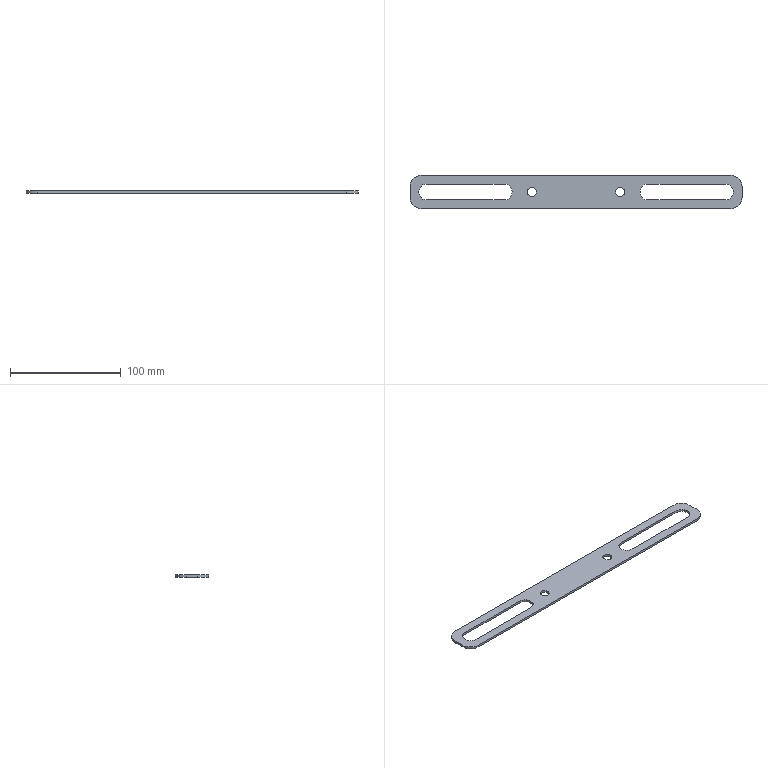Part | SolidWorks | features Fillet 2, ICE 2, Extrusion 1, MirrorPattern 1 | 1 solid | 24 faces | box 300 x 30 x 2 mm | volume 12944 mm3 | cylinder 14 | plane 10 | commonest cylinder face diameters 14.4 x6 8 x4 20 x4
STEP:
#1=CARTESIAN_POINT('',(44.,0.,2.));
#2=VERTEX_POINT('',#1);
#3=CARTESIAN_POINT('',(36.,0.,2.));
#4=VERTEX_POINT('',#3);
#5=CARTESIAN_POINT('',(40.,0.,2.));
#6=DIRECTION('',(0.,0.,-1.));
#7=DIRECTION('',(-1.,0.,0.));
#8=AXIS2_PLACEMENT_3D('',#5,#6,#7);
#9=CIRCLE('',#8,4.);
#10=EDGE_CURVE('',#2,#4,#9,.T.);
#11=ORIENTED_EDGE('',*,*,#10,.F.);
#12=CARTESIAN_POINT('',(44.,0.,0.));
#13=VERTEX_POINT('',#12);
#14=CARTESIAN_POINT('',(44.,0.,2.));
#15=DIRECTION('',(0.,0.,-1.));
#16=VECTOR('',#15,1000.);
#17=LINE('',#14,#16);
#18=EDGE_CURVE('',#2,#13,#17,.T.);
#19=ORIENTED_EDGE('',*,*,#18,.T.);
#20=CARTESIAN_POINT('',(36.,0.,0.));
#21=VERTEX_POINT('',#20);
#22=CARTESIAN_POINT('',(40.,0.,0.));
#23=DIRECTION('',(0.,0.,-1.));
#24=DIRECTION('',(-1.,0.,0.));
#25=AXIS2_PLACEMENT_3D('',#22,#23,#24);
#26=CIRCLE('',#25,4.);
#27=EDGE_CURVE('',#13,#21,#26,.T.);
#28=ORIENTED_EDGE('',*,*,#27,.T.);
#29=CARTESIAN_POINT('',(36.,0.,2.));
#30=DIRECTION('',(0.,0.,-1.));
#31=VECTOR('',#30,1000.);
#32=LINE('',#29,#31);
#33=EDGE_CURVE('',#4,#21,#32,.T.);
#34=ORIENTED_EDGE('',*,*,#33,.F.);
#35=EDGE_LOOP('',(#11,#19,#28,#34));
#36=FACE_OUTER_BOUND('',#35,.T.);
#37=CARTESIAN_POINT('',(40.,0.,2.));
#38=DIRECTION('',(0.,0.,-1.));
#39=DIRECTION('',(-1.,0.,0.));
#40=AXIS2_PLACEMENT_3D('',#37,#38,#39);
#41=CYLINDRICAL_SURFACE('',#40,4.);
#42=ADVANCED_FACE('',(#36),#41,.F.);
#43=CARTESIAN_POINT('',(-36.,0.,2.));
#44=VERTEX_POINT('',#43);
#45=CARTESIAN_POINT('',(-44.,0.,2.));
#46=VERTEX_POINT('',#45);
#47=CARTESIAN_POINT('',(-40.,0.,2.));
#48=DIRECTION('',(0.,0.,-1.));
#49=DIRECTION('',(-1.,0.,0.));
#50=AXIS2_PLACEMENT_3D('',#47,#48,#49);
#51=CIRCLE('',#50,4.);
#52=EDGE_CURVE('',#44,#46,#51,.T.);
#53=ORIENTED_EDGE('',*,*,#52,.F.);
#54=CARTESIAN_POINT('',(-36.,0.,0.));
#55=VERTEX_POINT('',#54);
#56=CARTESIAN_POINT('',(-36.,0.,2.));
#57=DIRECTION('',(0.,0.,-1.));
#58=VECTOR('',#57,1000.);
#59=LINE('',#56,#58);
#60=EDGE_CURVE('',#44,#55,#59,.T.);
#61=ORIENTED_EDGE('',*,*,#60,.T.);
#62=CARTESIAN_POINT('',(-44.,0.,0.));
#63=VERTEX_POINT('',#62);
#64=CARTESIAN_POINT('',(-40.,0.,0.));
#65=DIRECTION('',(0.,0.,-1.));
#66=DIRECTION('',(-1.,0.,0.));
#67=AXIS2_PLACEMENT_3D('',#64,#65,#66);
#68=CIRCLE('',#67,4.);
#69=EDGE_CURVE('',#55,#63,#68,.T.);
#70=ORIENTED_EDGE('',*,*,#69,.T.);
#71=CARTESIAN_POINT('',(-44.,0.,2.));
#72=DIRECTION('',(0.,0.,-1.));
#73=VECTOR('',#72,1000.);
#74=LINE('',#71,#73);
#75=EDGE_CURVE('',#46,#63,#74,.T.);
#76=ORIENTED_EDGE('',*,*,#75,.F.);
#77=EDGE_LOOP('',(#53,#61,#70,#76));
#78=FACE_OUTER_BOUND('',#77,.T.);
#79=CARTESIAN_POINT('',(-40.,0.,2.));
#80=DIRECTION('',(0.,0.,-1.));
#81=DIRECTION('',(-1.,0.,0.));
#82=AXIS2_PLACEMENT_3D('',#79,#80,#81);
#83=CYLINDRICAL_SURFACE('',#82,4.);
#84=ADVANCED_FACE('',(#78),#83,.F.);
#85=CARTESIAN_POINT('',(135.,7.2,0.));
#86=VERTEX_POINT('',#85);
#87=CARTESIAN_POINT('',(142.2,0.,0.));
#88=VERTEX_POINT('',#87);
#89=CARTESIAN_POINT('',(135.,0.,0.));
#90=DIRECTION('',(0.,0.,-1.));
#91=DIRECTION('',(-1.,0.,0.));
#92=AXIS2_PLACEMENT_3D('',#89,#90,#91);
#93=CIRCLE('',#92,7.2);
#94=EDGE_CURVE('',#86,#88,#93,.T.);
#95=ORIENTED_EDGE('',*,*,#94,.T.);
#96=CARTESIAN_POINT('',(142.2,0.,2.));
#97=VERTEX_POINT('',#96);
#98=CARTESIAN_POINT('',(142.2,0.,0.));
#99=DIRECTION('',(0.,0.,1.));
#100=VECTOR('',#99,1000.);
#101=LINE('',#98,#100);
#102=EDGE_CURVE('',#88,#97,#101,.T.);
#103=ORIENTED_EDGE('',*,*,#102,.T.);
#104=CARTESIAN_POINT('',(135.,7.2,2.));
#105=VERTEX_POINT('',#104);
#106=CARTESIAN_POINT('',(135.,0.,2.));
#107=DIRECTION('',(0.,0.,-1.));
#108=DIRECTION('',(-1.,0.,0.));
#109=AXIS2_PLACEMENT_3D('',#106,#107,#108);
#110=CIRCLE('',#109,7.2);
#111=EDGE_CURVE('',#105,#97,#110,.T.);
#112=ORIENTED_EDGE('',*,*,#111,.F.);
#113=CARTESIAN_POINT('',(135.,7.2,0.));
#114=DIRECTION('',(0.,0.,1.));
#115=VECTOR('',#114,1000.);
#116=LINE('',#113,#115);
#117=EDGE_CURVE('',#86,#105,#116,.T.);
#118=ORIENTED_EDGE('',*,*,#117,.F.);
#119=EDGE_LOOP('',(#95,#103,#112,#118));
#120=FACE_OUTER_BOUND('',#119,.T.);
#121=CARTESIAN_POINT('',(135.,0.,0.));
#122=DIRECTION('',(0.,0.,1.));
#123=DIRECTION('',(1.,0.,0.));
#124=AXIS2_PLACEMENT_3D('',#121,#122,#123);
#125=CYLINDRICAL_SURFACE('',#124,7.2);
#126=ADVANCED_FACE('',(#120),#125,.F.);
#127=CARTESIAN_POINT('',(-57.8,0.,0.));
#128=VERTEX_POINT('',#127);
#129=CARTESIAN_POINT('',(-65.,7.2,0.));
#130=VERTEX_POINT('',#129);
#131=CARTESIAN_POINT('',(-65.,0.,0.));
#132=DIRECTION('',(0.,0.,1.));
#133=DIRECTION('',(1.,0.,0.));
#134=AXIS2_PLACEMENT_3D('',#131,#132,#133);
#135=CIRCLE('',#134,7.2);
#136=EDGE_CURVE('',#128,#130,#135,.T.);
#137=ORIENTED_EDGE('',*,*,#136,.F.);
#138=CARTESIAN_POINT('',(-57.8,0.,2.));
#139=VERTEX_POINT('',#138);
#140=CARTESIAN_POINT('',(-57.8,0.,0.));
#141=DIRECTION('',(0.,0.,1.));
#142=VECTOR('',#141,1000.);
#143=LINE('',#140,#142);
#144=EDGE_CURVE('',#128,#139,#143,.T.);
#145=ORIENTED_EDGE('',*,*,#144,.T.);
#146=CARTESIAN_POINT('',(-65.,7.2,2.));
#147=VERTEX_POINT('',#146);
#148=CARTESIAN_POINT('',(-65.,0.,2.));
#149=DIRECTION('',(0.,0.,1.));
#150=DIRECTION('',(1.,0.,0.));
#151=AXIS2_PLACEMENT_3D('',#148,#149,#150);
#152=CIRCLE('',#151,7.2);
#153=EDGE_CURVE('',#139,#147,#152,.T.);
#154=ORIENTED_EDGE('',*,*,#153,.T.);
#155=CARTESIAN_POINT('',(-65.,7.2,0.));
#156=DIRECTION('',(0.,0.,1.));
#157=VECTOR('',#156,1000.);
#158=LINE('',#155,#157);
#159=EDGE_CURVE('',#130,#147,#158,.T.);
#160=ORIENTED_EDGE('',*,*,#159,.F.);
#161=EDGE_LOOP('',(#137,#145,#154,#160));
#162=FACE_OUTER_BOUND('',#161,.T.);
#163=CARTESIAN_POINT('',(-65.,0.,0.));
#164=DIRECTION('',(0.,0.,1.));
#165=DIRECTION('',(1.,0.,0.));
#166=AXIS2_PLACEMENT_3D('',#163,#164,#165);
#167=CYLINDRICAL_SURFACE('',#166,7.2);
#168=ADVANCED_FACE('',(#162),#167,.F.);
#169=CARTESIAN_POINT('',(40.,0.,2.));
#170=DIRECTION('',(0.,0.,-1.));
#171=DIRECTION('',(-1.,0.,0.));
#172=AXIS2_PLACEMENT_3D('',#169,#170,#171);
#173=CIRCLE('',#172,4.);
#174=EDGE_CURVE('',#4,#2,#173,.T.);
#175=ORIENTED_EDGE('',*,*,#174,.T.);
#176=ORIENTED_EDGE('',*,*,#10,.T.);
#177=EDGE_LOOP('',(#175,#176));
#178=FACE_BOUND('',#177,.T.);
#179=CARTESIAN_POINT('',(-40.,0.,2.));
#180=DIRECTION('',(0.,0.,-1.));
#181=DIRECTION('',(-1.,0.,0.));
#182=AXIS2_PLACEMENT_3D('',#179,#180,#181);
#183=CIRCLE('',#182,4.);
#184=EDGE_CURVE('',#46,#44,#183,.T.);
#185=ORIENTED_EDGE('',*,*,#184,.T.);
#186=ORIENTED_EDGE('',*,*,#52,.T.);
#187=EDGE_LOOP('',(#185,#186));
#188=FACE_BOUND('',#187,.T.);
#189=CARTESIAN_POINT('',(-140.,-15.,2.));
#190=VERTEX_POINT('',#189);
#191=CARTESIAN_POINT('',(140.,-15.,2.));
#192=VERTEX_POINT('',#191);
#193=CARTESIAN_POINT('',(150.,-15.,2.));
#194=DIRECTION('',(1.,0.,0.));
#195=VECTOR('',#194,1000.);
#196=LINE('',#193,#195);
#197=EDGE_CURVE('',#190,#192,#196,.T.);
#198=ORIENTED_EDGE('',*,*,#197,.T.);
#199=CARTESIAN_POINT('',(150.,-5.,2.));
#200=VERTEX_POINT('',#199);
#201=CARTESIAN_POINT('',(140.,-5.,2.));
#202=DIRECTION('',(0.,0.,1.));
#203=DIRECTION('',(1.,0.,0.));
#204=AXIS2_PLACEMENT_3D('',#201,#202,#203);
#205=CIRCLE('',#204,10.);
#206=EDGE_CURVE('',#192,#200,#205,.T.);
#207=ORIENTED_EDGE('',*,*,#206,.T.);
#208=CARTESIAN_POINT('',(150.,5.,2.));
#209=VERTEX_POINT('',#208);
#210=CARTESIAN_POINT('',(150.,-15.,2.));
#211=DIRECTION('',(0.,1.,0.));
#212=VECTOR('',#211,1000.);
#213=LINE('',#210,#212);
#214=EDGE_CURVE('',#200,#209,#213,.T.);
#215=ORIENTED_EDGE('',*,*,#214,.T.);
#216=CARTESIAN_POINT('',(140.,15.,2.));
#217=VERTEX_POINT('',#216);
#218=CARTESIAN_POINT('',(140.,5.,2.));
#219=DIRECTION('',(0.,0.,1.));
#220=DIRECTION('',(1.,0.,0.));
#221=AXIS2_PLACEMENT_3D('',#218,#219,#220);
#222=CIRCLE('',#221,10.);
#223=EDGE_CURVE('',#209,#217,#222,.T.);
#224=ORIENTED_EDGE('',*,*,#223,.T.);
#225=CARTESIAN_POINT('',(-140.,15.,2.));
#226=VERTEX_POINT('',#225);
#227=CARTESIAN_POINT('',(150.,15.,2.));
#228=DIRECTION('',(-1.,0.,0.));
#229=VECTOR('',#228,1000.);
#230=LINE('',#227,#229);
#231=EDGE_CURVE('',#217,#226,#230,.T.);
#232=ORIENTED_EDGE('',*,*,#231,.T.);
#233=CARTESIAN_POINT('',(-150.,5.,2.));
#234=VERTEX_POINT('',#233);
#235=CARTESIAN_POINT('',(-140.,5.,2.));
#236=DIRECTION('',(0.,0.,1.));
#237=DIRECTION('',(1.,0.,0.));
#238=AXIS2_PLACEMENT_3D('',#235,#236,#237);
#239=CIRCLE('',#238,10.);
#240=EDGE_CURVE('',#226,#234,#239,.T.);
#241=ORIENTED_EDGE('',*,*,#240,.T.);
#242=CARTESIAN_POINT('',(-150.,-5.,2.));
#243=VERTEX_POINT('',#242);
#244=CARTESIAN_POINT('',(-150.,-15.,2.));
#245=DIRECTION('',(0.,-1.,0.));
#246=VECTOR('',#245,1000.);
#247=LINE('',#244,#246);
#248=EDGE_CURVE('',#234,#243,#247,.T.);
#249=ORIENTED_EDGE('',*,*,#248,.T.);
#250=CARTESIAN_POINT('',(-140.,-5.,2.));
#251=DIRECTION('',(0.,0.,1.));
#252=DIRECTION('',(1.,0.,0.));
#253=AXIS2_PLACEMENT_3D('',#250,#251,#252);
#254=CIRCLE('',#253,10.);
#255=EDGE_CURVE('',#243,#190,#254,.T.);
#256=ORIENTED_EDGE('',*,*,#255,.T.);
#257=EDGE_LOOP('',(#198,#207,#215,#224,#232,#241,#249,#256));
#258=FACE_OUTER_BOUND('',#257,.T.);
#259=CARTESIAN_POINT('',(-135.,7.2,2.));
#260=VERTEX_POINT('',#259);
#261=CARTESIAN_POINT('',(-135.,-7.2,2.));
#262=VERTEX_POINT('',#261);
#263=CARTESIAN_POINT('',(-135.,0.,2.));
#264=DIRECTION('',(0.,0.,1.));
#265=DIRECTION('',(1.,0.,0.));
#266=AXIS2_PLACEMENT_3D('',#263,#264,#265);
#267=CIRCLE('',#266,7.2);
#268=EDGE_CURVE('',#260,#262,#267,.T.);
#269=ORIENTED_EDGE('',*,*,#268,.F.);
#270=CARTESIAN_POINT('',(-135.,7.2,2.));
#271=DIRECTION('',(-1.,0.,0.));
#272=VECTOR('',#271,1000.);
#273=LINE('',#270,#272);
#274=EDGE_CURVE('',#147,#260,#273,.T.);
#275=ORIENTED_EDGE('',*,*,#274,.F.);
#276=ORIENTED_EDGE('',*,*,#153,.F.);
#277=CARTESIAN_POINT('',(-65.,-7.2,2.));
#278=VERTEX_POINT('',#277);
#279=CARTESIAN_POINT('',(-65.,0.,2.));
#280=DIRECTION('',(0.,0.,1.));
#281=DIRECTION('',(1.,0.,0.));
#282=AXIS2_PLACEMENT_3D('',#279,#280,#281);
#283=CIRCLE('',#282,7.2);
#284=EDGE_CURVE('',#278,#139,#283,.T.);
#285=ORIENTED_EDGE('',*,*,#284,.F.);
#286=CARTESIAN_POINT('',(-135.,-7.2,2.));
#287=DIRECTION('',(1.,0.,0.));
#288=VECTOR('',#287,1000.);
#289=LINE('',#286,#288);
#290=EDGE_CURVE('',#262,#278,#289,.T.);
#291=ORIENTED_EDGE('',*,*,#290,.F.);
#292=EDGE_LOOP('',(#269,#275,#276,#285,#291));
#293=FACE_BOUND('',#292,.T.);
#294=CARTESIAN_POINT('',(65.,7.2,2.));
#295=VERTEX_POINT('',#294);
#296=CARTESIAN_POINT('',(135.,7.2,2.));
#297=DIRECTION('',(1.,0.,0.));
#298=VECTOR('',#297,1000.);
#299=LINE('',#296,#298);
#300=EDGE_CURVE('',#295,#105,#299,.T.);
#301=ORIENTED_EDGE('',*,*,#300,.T.);
#302=ORIENTED_EDGE('',*,*,#111,.T.);
#303=CARTESIAN_POINT('',(135.,-7.2,2.));
#304=VERTEX_POINT('',#303);
#305=CARTESIAN_POINT('',(135.,0.,2.));
#306=DIRECTION('',(0.,0.,-1.));
#307=DIRECTION('',(-1.,0.,0.));
#308=AXIS2_PLACEMENT_3D('',#305,#306,#307);
#309=CIRCLE('',#308,7.2);
#310=EDGE_CURVE('',#97,#304,#309,.T.);
#311=ORIENTED_EDGE('',*,*,#310,.T.);
#312=CARTESIAN_POINT('',(65.,-7.2,2.));
#313=VERTEX_POINT('',#312);
#314=CARTESIAN_POINT('',(135.,-7.2,2.));
#315=DIRECTION('',(-1.,0.,0.));
#316=VECTOR('',#315,1000.);
#317=LINE('',#314,#316);
#318=EDGE_CURVE('',#304,#313,#317,.T.);
#319=ORIENTED_EDGE('',*,*,#318,.T.);
#320=CARTESIAN_POINT('',(65.,0.,2.));
#321=DIRECTION('',(0.,0.,-1.));
#322=DIRECTION('',(-1.,0.,0.));
#323=AXIS2_PLACEMENT_3D('',#320,#321,#322);
#324=CIRCLE('',#323,7.2);
#325=EDGE_CURVE('',#313,#295,#324,.T.);
#326=ORIENTED_EDGE('',*,*,#325,.T.);
#327=EDGE_LOOP('',(#301,#302,#311,#319,#326));
#328=FACE_BOUND('',#327,.T.);
#329=CARTESIAN_POINT('',(0.,0.,2.));
#330=DIRECTION('',(0.,0.,1.));
#331=DIRECTION('',(1.,0.,0.));
#332=AXIS2_PLACEMENT_3D('',#329,#330,#331);
#333=PLANE('',#332);
#334=ADVANCED_FACE('',(#178,#188,#258,#293,#328),#333,.T.);
#335=CARTESIAN_POINT('',(40.,0.,0.));
#336=DIRECTION('',(0.,0.,-1.));
#337=DIRECTION('',(-1.,0.,0.));
#338=AXIS2_PLACEMENT_3D('',#335,#336,#337);
#339=CIRCLE('',#338,4.);
#340=EDGE_CURVE('',#21,#13,#339,.T.);
#341=ORIENTED_EDGE('',*,*,#340,.F.);
#342=ORIENTED_EDGE('',*,*,#27,.F.);
#343=EDGE_LOOP('',(#341,#342));
#344=FACE_BOUND('',#343,.T.);
#345=CARTESIAN_POINT('',(-40.,0.,0.));
#346=DIRECTION('',(0.,0.,-1.));
#347=DIRECTION('',(-1.,0.,0.));
#348=AXIS2_PLACEMENT_3D('',#345,#346,#347);
#349=CIRCLE('',#348,4.);
#350=EDGE_CURVE('',#63,#55,#349,.T.);
#351=ORIENTED_EDGE('',*,*,#350,.F.);
#352=ORIENTED_EDGE('',*,*,#69,.F.);
#353=EDGE_LOOP('',(#351,#352));
#354=FACE_BOUND('',#353,.T.);
#355=CARTESIAN_POINT('',(150.,-5.,0.));
#356=VERTEX_POINT('',#355);
#357=CARTESIAN_POINT('',(150.,5.,0.));
#358=VERTEX_POINT('',#357);
#359=CARTESIAN_POINT('',(150.,-15.,0.));
#360=DIRECTION('',(0.,1.,0.));
#361=VECTOR('',#360,1000.);
#362=LINE('',#359,#361);
#363=EDGE_CURVE('',#356,#358,#362,.T.);
#364=ORIENTED_EDGE('',*,*,#363,.F.);
#365=CARTESIAN_POINT('',(140.,-15.,0.));
#366=VERTEX_POINT('',#365);
#367=CARTESIAN_POINT('',(140.,-5.,0.));
#368=DIRECTION('',(0.,0.,-1.));
#369=DIRECTION('',(1.,0.,0.));
#370=AXIS2_PLACEMENT_3D('',#367,#368,#369);
#371=CIRCLE('',#370,10.);
#372=EDGE_CURVE('',#356,#366,#371,.T.);
#373=ORIENTED_EDGE('',*,*,#372,.T.);
#374=CARTESIAN_POINT('',(-140.,-15.,0.));
#375=VERTEX_POINT('',#374);
#376=CARTESIAN_POINT('',(150.,-15.,0.));
#377=DIRECTION('',(1.,0.,0.));
#378=VECTOR('',#377,1000.);
#379=LINE('',#376,#378);
#380=EDGE_CURVE('',#375,#366,#379,.T.);
#381=ORIENTED_EDGE('',*,*,#380,.F.);
#382=CARTESIAN_POINT('',(-150.,-5.,0.));
#383=VERTEX_POINT('',#382);
#384=CARTESIAN_POINT('',(-140.,-5.,0.));
#385=DIRECTION('',(0.,0.,-1.));
#386=DIRECTION('',(1.,0.,0.));
#387=AXIS2_PLACEMENT_3D('',#384,#385,#386);
#388=CIRCLE('',#387,10.);
#389=EDGE_CURVE('',#375,#383,#388,.T.);
#390=ORIENTED_EDGE('',*,*,#389,.T.);
#391=CARTESIAN_POINT('',(-150.,5.,0.));
#392=VERTEX_POINT('',#391);
#393=CARTESIAN_POINT('',(-150.,-15.,0.));
#394=DIRECTION('',(0.,-1.,0.));
#395=VECTOR('',#394,1000.);
#396=LINE('',#393,#395);
#397=EDGE_CURVE('',#392,#383,#396,.T.);
#398=ORIENTED_EDGE('',*,*,#397,.F.);
#399=CARTESIAN_POINT('',(-140.,15.,0.));
#400=VERTEX_POINT('',#399);
#401=CARTESIAN_POINT('',(-140.,5.,0.));
#402=DIRECTION('',(0.,0.,-1.));
#403=DIRECTION('',(1.,0.,0.));
#404=AXIS2_PLACEMENT_3D('',#401,#402,#403);
#405=CIRCLE('',#404,10.);
#406=EDGE_CURVE('',#392,#400,#405,.T.);
#407=ORIENTED_EDGE('',*,*,#406,.T.);
#408=CARTESIAN_POINT('',(140.,15.,0.));
#409=VERTEX_POINT('',#408);
#410=CARTESIAN_POINT('',(150.,15.,0.));
#411=DIRECTION('',(-1.,0.,0.));
#412=VECTOR('',#411,1000.);
#413=LINE('',#410,#412);
#414=EDGE_CURVE('',#409,#400,#413,.T.);
#415=ORIENTED_EDGE('',*,*,#414,.F.);
#416=CARTESIAN_POINT('',(140.,5.,0.));
#417=DIRECTION('',(0.,0.,-1.));
#418=DIRECTION('',(1.,0.,0.));
#419=AXIS2_PLACEMENT_3D('',#416,#417,#418);
#420=CIRCLE('',#419,10.);
#421=EDGE_CURVE('',#409,#358,#420,.T.);
#422=ORIENTED_EDGE('',*,*,#421,.T.);
#423=EDGE_LOOP('',(#364,#373,#381,#390,#398,#407,#415,#422));
#424=FACE_OUTER_BOUND('',#423,.T.);
#425=CARTESIAN_POINT('',(-135.,7.2,0.));
#426=VERTEX_POINT('',#425);
#427=CARTESIAN_POINT('',(-135.,7.2,0.));
#428=DIRECTION('',(-1.,0.,0.));
#429=VECTOR('',#428,1000.);
#430=LINE('',#427,#429);
#431=EDGE_CURVE('',#130,#426,#430,.T.);
#432=ORIENTED_EDGE('',*,*,#431,.T.);
#433=CARTESIAN_POINT('',(-135.,-7.2,0.));
#434=VERTEX_POINT('',#433);
#435=CARTESIAN_POINT('',(-135.,0.,0.));
#436=DIRECTION('',(0.,0.,1.));
#437=DIRECTION('',(1.,0.,0.));
#438=AXIS2_PLACEMENT_3D('',#435,#436,#437);
#439=CIRCLE('',#438,7.2);
#440=EDGE_CURVE('',#426,#434,#439,.T.);
#441=ORIENTED_EDGE('',*,*,#440,.T.);
#442=CARTESIAN_POINT('',(-65.,-7.2,0.));
#443=VERTEX_POINT('',#442);
#444=CARTESIAN_POINT('',(-135.,-7.2,0.));
#445=DIRECTION('',(1.,0.,0.));
#446=VECTOR('',#445,1000.);
#447=LINE('',#444,#446);
#448=EDGE_CURVE('',#434,#443,#447,.T.);
#449=ORIENTED_EDGE('',*,*,#448,.T.);
#450=CARTESIAN_POINT('',(-65.,0.,0.));
#451=DIRECTION('',(0.,0.,1.));
#452=DIRECTION('',(1.,0.,0.));
#453=AXIS2_PLACEMENT_3D('',#450,#451,#452);
#454=CIRCLE('',#453,7.2);
#455=EDGE_CURVE('',#443,#128,#454,.T.);
#456=ORIENTED_EDGE('',*,*,#455,.T.);
#457=ORIENTED_EDGE('',*,*,#136,.T.);
#458=EDGE_LOOP('',(#432,#441,#449,#456,#457));
#459=FACE_BOUND('',#458,.T.);
#460=ORIENTED_EDGE('',*,*,#94,.F.);
#461=CARTESIAN_POINT('',(65.,7.2,0.));
#462=VERTEX_POINT('',#461);
#463=CARTESIAN_POINT('',(135.,7.2,0.));
#464=DIRECTION('',(1.,0.,0.));
#465=VECTOR('',#464,1000.);
#466=LINE('',#463,#465);
#467=EDGE_CURVE('',#462,#86,#466,.T.);
#468=ORIENTED_EDGE('',*,*,#467,.F.);
#469=CARTESIAN_POINT('',(65.,-7.2,0.));
#470=VERTEX_POINT('',#469);
#471=CARTESIAN_POINT('',(65.,0.,0.));
#472=DIRECTION('',(0.,0.,-1.));
#473=DIRECTION('',(-1.,0.,0.));
#474=AXIS2_PLACEMENT_3D('',#471,#472,#473);
#475=CIRCLE('',#474,7.2);
#476=EDGE_CURVE('',#470,#462,#475,.T.);
#477=ORIENTED_EDGE('',*,*,#476,.F.);
#478=CARTESIAN_POINT('',(135.,-7.2,0.));
#479=VERTEX_POINT('',#478);
#480=CARTESIAN_POINT('',(135.,-7.2,0.));
#481=DIRECTION('',(-1.,0.,0.));
#482=VECTOR('',#481,1000.);
#483=LINE('',#480,#482);
#484=EDGE_CURVE('',#479,#470,#483,.T.);
#485=ORIENTED_EDGE('',*,*,#484,.F.);
#486=CARTESIAN_POINT('',(135.,0.,0.));
#487=DIRECTION('',(0.,0.,-1.));
#488=DIRECTION('',(-1.,0.,0.));
#489=AXIS2_PLACEMENT_3D('',#486,#487,#488);
#490=CIRCLE('',#489,7.2);
#491=EDGE_CURVE('',#88,#479,#490,.T.);
#492=ORIENTED_EDGE('',*,*,#491,.F.);
#493=EDGE_LOOP('',(#460,#468,#477,#485,#492));
#494=FACE_BOUND('',#493,.T.);
#495=CARTESIAN_POINT('',(0.,0.,0.));
#496=DIRECTION('',(0.,0.,1.));
#497=DIRECTION('',(1.,0.,0.));
#498=AXIS2_PLACEMENT_3D('',#495,#496,#497);
#499=PLANE('',#498);
#500=ADVANCED_FACE('',(#344,#354,#424,#459,#494),#499,.F.);
#501=ORIENTED_EDGE('',*,*,#248,.F.);
#502=CARTESIAN_POINT('',(-150.,5.,2.));
#503=DIRECTION('',(0.,0.,-1.));
#504=VECTOR('',#503,1000.);
#505=LINE('',#502,#504);
#506=EDGE_CURVE('',#234,#392,#505,.T.);
#507=ORIENTED_EDGE('',*,*,#506,.T.);
#508=ORIENTED_EDGE('',*,*,#397,.T.);
#509=CARTESIAN_POINT('',(-150.,-5.,2.));
#510=DIRECTION('',(0.,0.,1.));
#511=VECTOR('',#510,1000.);
#512=LINE('',#509,#511);
#513=EDGE_CURVE('',#383,#243,#512,.T.);
#514=ORIENTED_EDGE('',*,*,#513,.T.);
#515=EDGE_LOOP('',(#501,#507,#508,#514));
#516=FACE_OUTER_BOUND('',#515,.T.);
#517=CARTESIAN_POINT('',(-150.,-15.,2.));
#518=DIRECTION('',(1.,0.,0.));
#519=DIRECTION('',(0.,0.,-1.));
#520=AXIS2_PLACEMENT_3D('',#517,#518,#519);
#521=PLANE('',#520);
#522=ADVANCED_FACE('',(#516),#521,.F.);
#523=ORIENTED_EDGE('',*,*,#380,.T.);
#524=CARTESIAN_POINT('',(140.,-15.,2.));
#525=DIRECTION('',(0.,0.,1.));
#526=VECTOR('',#525,1000.);
#527=LINE('',#524,#526);
#528=EDGE_CURVE('',#366,#192,#527,.T.);
#529=ORIENTED_EDGE('',*,*,#528,.T.);
#530=ORIENTED_EDGE('',*,*,#197,.F.);
#531=CARTESIAN_POINT('',(-140.,-15.,2.));
#532=DIRECTION('',(0.,0.,-1.));
#533=VECTOR('',#532,1000.);
#534=LINE('',#531,#533);
#535=EDGE_CURVE('',#190,#375,#534,.T.);
#536=ORIENTED_EDGE('',*,*,#535,.T.);
#537=EDGE_LOOP('',(#523,#529,#530,#536));
#538=FACE_OUTER_BOUND('',#537,.T.);
#539=CARTESIAN_POINT('',(150.,-15.,2.));
#540=DIRECTION('',(0.,1.,0.));
#541=DIRECTION('',(-1.,0.,0.));
#542=AXIS2_PLACEMENT_3D('',#539,#540,#541);
#543=PLANE('',#542);
#544=ADVANCED_FACE('',(#538),#543,.F.);
#545=ORIENTED_EDGE('',*,*,#214,.F.);
#546=CARTESIAN_POINT('',(150.,-5.,2.));
#547=DIRECTION('',(0.,0.,-1.));
#548=VECTOR('',#547,1000.);
#549=LINE('',#546,#548);
#550=EDGE_CURVE('',#200,#356,#549,.T.);
#551=ORIENTED_EDGE('',*,*,#550,.T.);
#552=ORIENTED_EDGE('',*,*,#363,.T.);
#553=CARTESIAN_POINT('',(150.,5.,2.));
#554=DIRECTION('',(0.,0.,1.));
#555=VECTOR('',#554,1000.);
#556=LINE('',#553,#555);
#557=EDGE_CURVE('',#358,#209,#556,.T.);
#558=ORIENTED_EDGE('',*,*,#557,.T.);
#559=EDGE_LOOP('',(#545,#551,#552,#558));
#560=FACE_OUTER_BOUND('',#559,.T.);
#561=CARTESIAN_POINT('',(150.,-15.,2.));
#562=DIRECTION('',(-1.,0.,0.));
#563=DIRECTION('',(0.,0.,1.));
#564=AXIS2_PLACEMENT_3D('',#561,#562,#563);
#565=PLANE('',#564);
#566=ADVANCED_FACE('',(#560),#565,.F.);
#567=ORIENTED_EDGE('',*,*,#231,.F.);
#568=CARTESIAN_POINT('',(140.,15.,2.));
#569=DIRECTION('',(0.,0.,-1.));
#570=VECTOR('',#569,1000.);
#571=LINE('',#568,#570);
#572=EDGE_CURVE('',#217,#409,#571,.T.);
#573=ORIENTED_EDGE('',*,*,#572,.T.);
#574=ORIENTED_EDGE('',*,*,#414,.T.);
#575=CARTESIAN_POINT('',(-140.,15.,2.));
#576=DIRECTION('',(0.,0.,1.));
#577=VECTOR('',#576,1000.);
#578=LINE('',#575,#577);
#579=EDGE_CURVE('',#400,#226,#578,.T.);
#580=ORIENTED_EDGE('',*,*,#579,.T.);
#581=EDGE_LOOP('',(#567,#573,#574,#580));
#582=FACE_OUTER_BOUND('',#581,.T.);
#583=CARTESIAN_POINT('',(150.,15.,2.));
#584=DIRECTION('',(0.,-1.,0.));
#585=DIRECTION('',(1.,0.,0.));
#586=AXIS2_PLACEMENT_3D('',#583,#584,#585);
#587=PLANE('',#586);
#588=ADVANCED_FACE('',(#582),#587,.F.);
#589=ORIENTED_EDGE('',*,*,#268,.T.);
#590=CARTESIAN_POINT('',(-135.,-7.2,0.));
#591=DIRECTION('',(0.,0.,1.));
#592=VECTOR('',#591,1000.);
#593=LINE('',#590,#592);
#594=EDGE_CURVE('',#434,#262,#593,.T.);
#595=ORIENTED_EDGE('',*,*,#594,.F.);
#596=ORIENTED_EDGE('',*,*,#440,.F.);
#597=CARTESIAN_POINT('',(-135.,7.2,0.));
#598=DIRECTION('',(0.,0.,1.));
#599=VECTOR('',#598,1000.);
#600=LINE('',#597,#599);
#601=EDGE_CURVE('',#426,#260,#600,.T.);
#602=ORIENTED_EDGE('',*,*,#601,.T.);
#603=EDGE_LOOP('',(#589,#595,#596,#602));
#604=FACE_OUTER_BOUND('',#603,.T.);
#605=CARTESIAN_POINT('',(-135.,0.,0.));
#606=DIRECTION('',(0.,0.,1.));
#607=DIRECTION('',(1.,0.,0.));
#608=AXIS2_PLACEMENT_3D('',#605,#606,#607);
#609=CYLINDRICAL_SURFACE('',#608,7.2);
#610=ADVANCED_FACE('',(#604),#609,.F.);
#611=ORIENTED_EDGE('',*,*,#274,.T.);
#612=ORIENTED_EDGE('',*,*,#601,.F.);
#613=ORIENTED_EDGE('',*,*,#431,.F.);
#614=ORIENTED_EDGE('',*,*,#159,.T.);
#615=EDGE_LOOP('',(#611,#612,#613,#614));
#616=FACE_OUTER_BOUND('',#615,.T.);
#617=CARTESIAN_POINT('',(-135.,7.2,0.));
#618=DIRECTION('',(0.,1.,0.));
#619=DIRECTION('',(-1.,0.,0.));
#620=AXIS2_PLACEMENT_3D('',#617,#618,#619);
#621=PLANE('',#620);
#622=ADVANCED_FACE('',(#616),#621,.F.);
#623=ORIENTED_EDGE('',*,*,#144,.F.);
#624=ORIENTED_EDGE('',*,*,#455,.F.);
#625=CARTESIAN_POINT('',(-65.,-7.2,0.));
#626=DIRECTION('',(0.,0.,1.));
#627=VECTOR('',#626,1000.);
#628=LINE('',#625,#627);
#629=EDGE_CURVE('',#443,#278,#628,.T.);
#630=ORIENTED_EDGE('',*,*,#629,.T.);
#631=ORIENTED_EDGE('',*,*,#284,.T.);
#632=EDGE_LOOP('',(#623,#624,#630,#631));
#633=FACE_OUTER_BOUND('',#632,.T.);
#634=CARTESIAN_POINT('',(-65.,0.,0.));
#635=DIRECTION('',(0.,0.,1.));
#636=DIRECTION('',(1.,0.,0.));
#637=AXIS2_PLACEMENT_3D('',#634,#635,#636);
#638=CYLINDRICAL_SURFACE('',#637,7.2);
#639=ADVANCED_FACE('',(#633),#638,.F.);
#640=ORIENTED_EDGE('',*,*,#290,.T.);
#641=ORIENTED_EDGE('',*,*,#629,.F.);
#642=ORIENTED_EDGE('',*,*,#448,.F.);
#643=ORIENTED_EDGE('',*,*,#594,.T.);
#644=EDGE_LOOP('',(#640,#641,#642,#643));
#645=FACE_OUTER_BOUND('',#644,.T.);
#646=CARTESIAN_POINT('',(-135.,-7.2,0.));
#647=DIRECTION('',(0.,-1.,0.));
#648=DIRECTION('',(1.,0.,0.));
#649=AXIS2_PLACEMENT_3D('',#646,#647,#648);
#650=PLANE('',#649);
#651=ADVANCED_FACE('',(#645),#650,.F.);
#652=ORIENTED_EDGE('',*,*,#240,.F.);
#653=ORIENTED_EDGE('',*,*,#579,.F.);
#654=ORIENTED_EDGE('',*,*,#406,.F.);
#655=ORIENTED_EDGE('',*,*,#506,.F.);
#656=EDGE_LOOP('',(#652,#653,#654,#655));
#657=FACE_OUTER_BOUND('',#656,.T.);
#658=CARTESIAN_POINT('',(-140.,5.,2.));
#659=DIRECTION('',(0.,0.,-1.));
#660=DIRECTION('',(-1.,0.,0.));
#661=AXIS2_PLACEMENT_3D('',#658,#659,#660);
#662=CYLINDRICAL_SURFACE('',#661,10.);
#663=ADVANCED_FACE('',(#657),#662,.T.);
#664=ORIENTED_EDGE('',*,*,#255,.F.);
#665=ORIENTED_EDGE('',*,*,#513,.F.);
#666=ORIENTED_EDGE('',*,*,#389,.F.);
#667=ORIENTED_EDGE('',*,*,#535,.F.);
#668=EDGE_LOOP('',(#664,#665,#666,#667));
#669=FACE_OUTER_BOUND('',#668,.T.);
#670=CARTESIAN_POINT('',(-140.,-5.,2.));
#671=DIRECTION('',(0.,0.,-1.));
#672=DIRECTION('',(-1.,0.,0.));
#673=AXIS2_PLACEMENT_3D('',#670,#671,#672);
#674=CYLINDRICAL_SURFACE('',#673,10.);
#675=ADVANCED_FACE('',(#669),#674,.T.);
#676=ORIENTED_EDGE('',*,*,#102,.F.);
#677=ORIENTED_EDGE('',*,*,#491,.T.);
#678=CARTESIAN_POINT('',(135.,-7.2,0.));
#679=DIRECTION('',(0.,0.,1.));
#680=VECTOR('',#679,1000.);
#681=LINE('',#678,#680);
#682=EDGE_CURVE('',#479,#304,#681,.T.);
#683=ORIENTED_EDGE('',*,*,#682,.T.);
#684=ORIENTED_EDGE('',*,*,#310,.F.);
#685=EDGE_LOOP('',(#676,#677,#683,#684));
#686=FACE_OUTER_BOUND('',#685,.T.);
#687=CARTESIAN_POINT('',(135.,0.,0.));
#688=DIRECTION('',(0.,0.,1.));
#689=DIRECTION('',(1.,0.,0.));
#690=AXIS2_PLACEMENT_3D('',#687,#688,#689);
#691=CYLINDRICAL_SURFACE('',#690,7.2);
#692=ADVANCED_FACE('',(#686),#691,.F.);
#693=ORIENTED_EDGE('',*,*,#318,.F.);
#694=ORIENTED_EDGE('',*,*,#682,.F.);
#695=ORIENTED_EDGE('',*,*,#484,.T.);
#696=CARTESIAN_POINT('',(65.,-7.2,0.));
#697=DIRECTION('',(0.,0.,1.));
#698=VECTOR('',#697,1000.);
#699=LINE('',#696,#698);
#700=EDGE_CURVE('',#470,#313,#699,.T.);
#701=ORIENTED_EDGE('',*,*,#700,.T.);
#702=EDGE_LOOP('',(#693,#694,#695,#701));
#703=FACE_OUTER_BOUND('',#702,.T.);
#704=CARTESIAN_POINT('',(135.,-7.2,0.));
#705=DIRECTION('',(0.,1.,0.));
#706=DIRECTION('',(-1.,0.,0.));
#707=AXIS2_PLACEMENT_3D('',#704,#705,#706);
#708=PLANE('',#707);
#709=ADVANCED_FACE('',(#703),#708,.T.);
#710=ORIENTED_EDGE('',*,*,#325,.F.);
#711=ORIENTED_EDGE('',*,*,#700,.F.);
#712=ORIENTED_EDGE('',*,*,#476,.T.);
#713=CARTESIAN_POINT('',(65.,7.2,0.));
#714=DIRECTION('',(0.,0.,1.));
#715=VECTOR('',#714,1000.);
#716=LINE('',#713,#715);
#717=EDGE_CURVE('',#462,#295,#716,.T.);
#718=ORIENTED_EDGE('',*,*,#717,.T.);
#719=EDGE_LOOP('',(#710,#711,#712,#718));
#720=FACE_OUTER_BOUND('',#719,.T.);
#721=CARTESIAN_POINT('',(65.,0.,0.));
#722=DIRECTION('',(0.,0.,1.));
#723=DIRECTION('',(1.,0.,0.));
#724=AXIS2_PLACEMENT_3D('',#721,#722,#723);
#725=CYLINDRICAL_SURFACE('',#724,7.2);
#726=ADVANCED_FACE('',(#720),#725,.F.);
#727=ORIENTED_EDGE('',*,*,#300,.F.);
#728=ORIENTED_EDGE('',*,*,#717,.F.);
#729=ORIENTED_EDGE('',*,*,#467,.T.);
#730=ORIENTED_EDGE('',*,*,#117,.T.);
#731=EDGE_LOOP('',(#727,#728,#729,#730));
#732=FACE_OUTER_BOUND('',#731,.T.);
#733=CARTESIAN_POINT('',(135.,7.2,0.));
#734=DIRECTION('',(0.,-1.,0.));
#735=DIRECTION('',(1.,0.,0.));
#736=AXIS2_PLACEMENT_3D('',#733,#734,#735);
#737=PLANE('',#736);
#738=ADVANCED_FACE('',(#732),#737,.T.);
#739=ORIENTED_EDGE('',*,*,#206,.F.);
#740=ORIENTED_EDGE('',*,*,#528,.F.);
#741=ORIENTED_EDGE('',*,*,#372,.F.);
#742=ORIENTED_EDGE('',*,*,#550,.F.);
#743=EDGE_LOOP('',(#739,#740,#741,#742));
#744=FACE_OUTER_BOUND('',#743,.T.);
#745=CARTESIAN_POINT('',(140.,-5.,2.));
#746=DIRECTION('',(0.,0.,-1.));
#747=DIRECTION('',(-1.,0.,0.));
#748=AXIS2_PLACEMENT_3D('',#745,#746,#747);
#749=CYLINDRICAL_SURFACE('',#748,10.);
#750=ADVANCED_FACE('',(#744),#749,.T.);
#751=ORIENTED_EDGE('',*,*,#223,.F.);
#752=ORIENTED_EDGE('',*,*,#557,.F.);
#753=ORIENTED_EDGE('',*,*,#421,.F.);
#754=ORIENTED_EDGE('',*,*,#572,.F.);
#755=EDGE_LOOP('',(#751,#752,#753,#754));
#756=FACE_OUTER_BOUND('',#755,.T.);
#757=CARTESIAN_POINT('',(140.,5.,2.));
#758=DIRECTION('',(0.,0.,-1.));
#759=DIRECTION('',(-1.,0.,0.));
#760=AXIS2_PLACEMENT_3D('',#757,#758,#759);
#761=CYLINDRICAL_SURFACE('',#760,10.);
#762=ADVANCED_FACE('',(#756),#761,.T.);
#763=ORIENTED_EDGE('',*,*,#60,.F.);
#764=ORIENTED_EDGE('',*,*,#184,.F.);
#765=ORIENTED_EDGE('',*,*,#75,.T.);
#766=ORIENTED_EDGE('',*,*,#350,.T.);
#767=EDGE_LOOP('',(#763,#764,#765,#766));
#768=FACE_OUTER_BOUND('',#767,.T.);
#769=CARTESIAN_POINT('',(-40.,0.,2.));
#770=DIRECTION('',(0.,0.,-1.));
#771=DIRECTION('',(-1.,0.,0.));
#772=AXIS2_PLACEMENT_3D('',#769,#770,#771);
#773=CYLINDRICAL_SURFACE('',#772,4.);
#774=ADVANCED_FACE('',(#768),#773,.F.);
#775=ORIENTED_EDGE('',*,*,#18,.F.);
#776=ORIENTED_EDGE('',*,*,#174,.F.);
#777=ORIENTED_EDGE('',*,*,#33,.T.);
#778=ORIENTED_EDGE('',*,*,#340,.T.);
#779=EDGE_LOOP('',(#775,#776,#777,#778));
#780=FACE_OUTER_BOUND('',#779,.T.);
#781=CARTESIAN_POINT('',(40.,0.,2.));
#782=DIRECTION('',(0.,0.,-1.));
#783=DIRECTION('',(-1.,0.,0.));
#784=AXIS2_PLACEMENT_3D('',#781,#782,#783);
#785=CYLINDRICAL_SURFACE('',#784,4.);
#786=ADVANCED_FACE('',(#780),#785,.F.);
#787=CLOSED_SHELL('',(#42,#84,#126,#168,#334,#500,#522,#544,#566,#588,#610,#622,#639,#651,#663,#675,#692,#709,#726,#738,#750,#762,#774,#786));
#788=MANIFOLD_SOLID_BREP('',#787);
#789=CARTESIAN_POINT('',(0.,0.,0.));
#790=DIRECTION('',(0.,0.,1.));
#791=DIRECTION('',(1.,0.,0.));
#792=AXIS2_PLACEMENT_3D('',#789,#790,#791);
#793=(LENGTH_UNIT()NAMED_UNIT(*)SI_UNIT(.MILLI.,.METRE.));
#794=UNCERTAINTY_MEASURE_WITH_UNIT(LENGTH_MEASURE(0.00001),#793,'','');
#795=(NAMED_UNIT(*)PLANE_ANGLE_UNIT()SI_UNIT($,.RADIAN.));
#796=(NAMED_UNIT(*)SI_UNIT($,.STERADIAN.)SOLID_ANGLE_UNIT());
#797=(GEOMETRIC_REPRESENTATION_CONTEXT(3)GLOBAL_UNCERTAINTY_ASSIGNED_CONTEXT((#794))GLOBAL_UNIT_ASSIGNED_CONTEXT((#793,#795,#796))REPRESENTATION_CONTEXT('',''));
#798=ADVANCED_BREP_SHAPE_REPRESENTATION('',(#788,#792),#797);